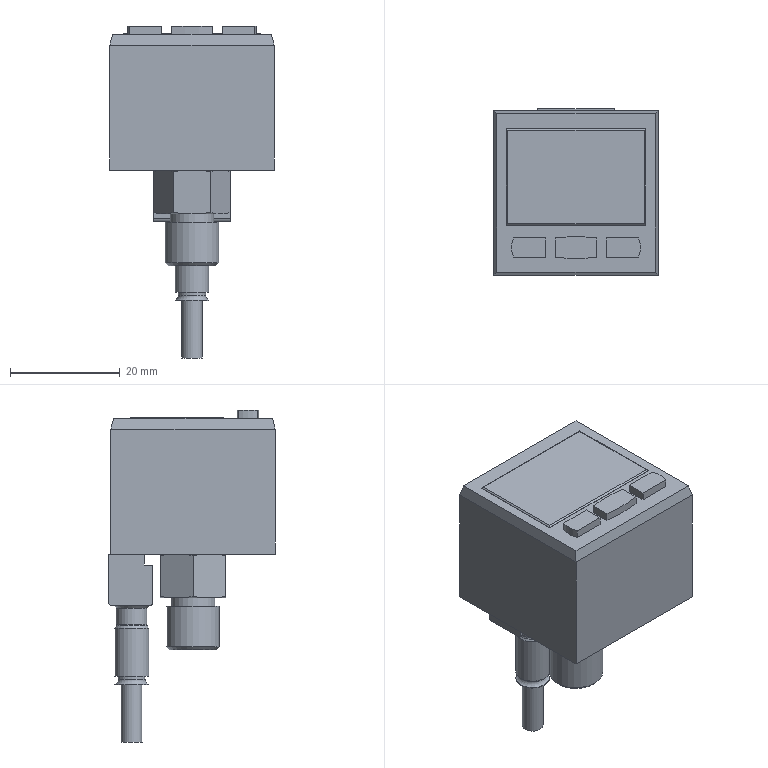Part | NX | 1 solid | 124 faces | box 30 x 30.38 x 60.6 mm | volume 25400 mm3 | plane 75 | cone 27 | cylinder 20 | torus 2 | commonest cylinder face diameters 1 x2 2.459 x2 2.6 x2 4 x2 9 x2 56.5 x2